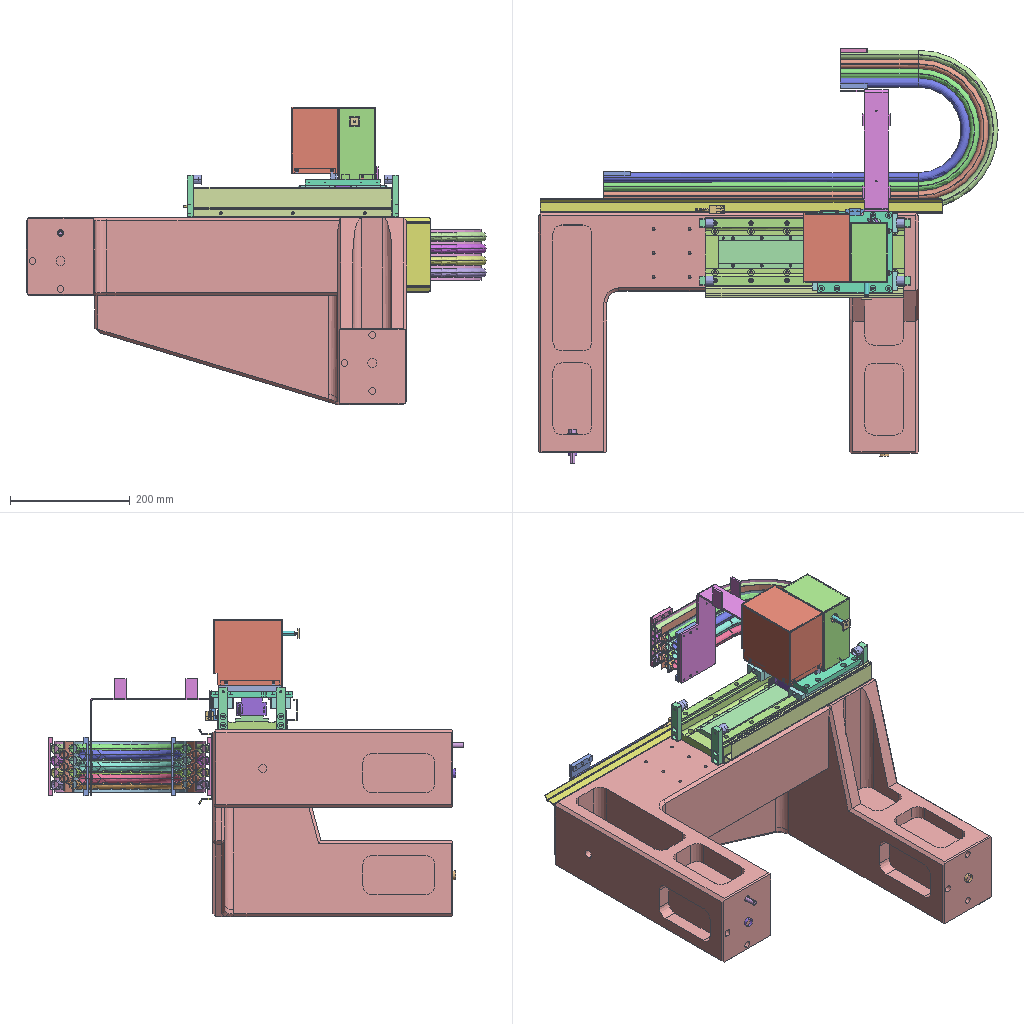Assembly | STEP file | 70 different items | 103 placed | box 767 x 693 x 496 mm
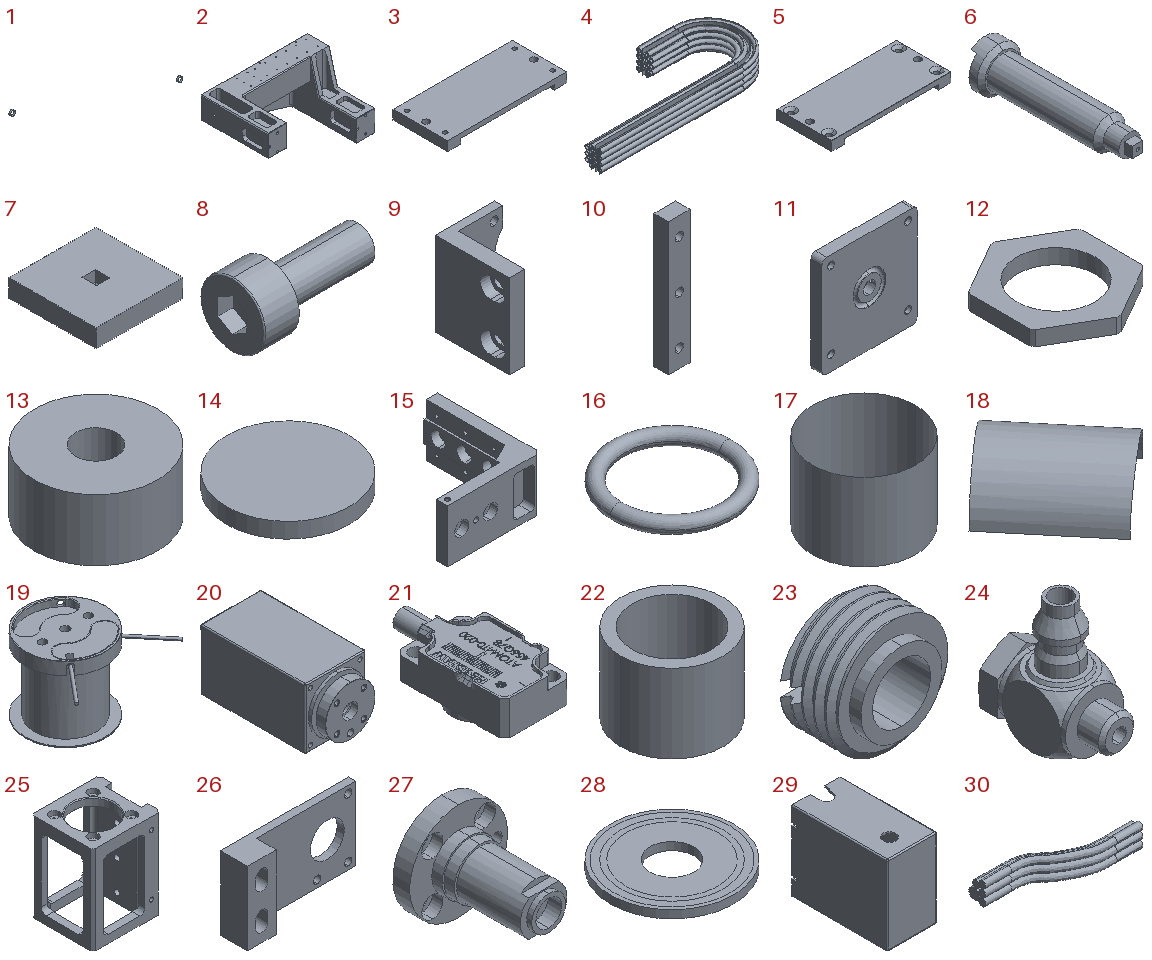Parts list (item | name | quantity | size | volume):
1 | COMPOUND | x1 | - | -
2 | SOLID | x1 | 635 x 400 x 312 mm | 15425228 mm3
3 | - | x2 | 97.7 x 44.7 x 7.7 mm | 19346 mm3
4 | - | x1 | 658 x 266 x 85.182 mm | 995637 mm3
5 | - | x2 | 97.7 x 44.7 x 7.7 mm | 18958 mm3
6 | - | x1 | 11 x 38.5 x 11 mm | 1504 mm3
7 | - | x1 | 16 x 16 x 3.3 mm | 788.101 mm3
8 | - | x1 | 11 x 5.5 x 5.5 mm | 120.454 mm3
9 | - | x1 | 14.8 x 18.5 x 21 mm | 1569 mm3
10 | - | x2 | 9 x 6 x 55 mm | 2652 mm3
11 | - | x1 | 39 x 10 x 41.5 mm | 7133 mm3
12 | - | x1 | 15 x 17 x 2 mm | 215.987 mm3
13 | - | x1 | 6 x 6 x 3 mm | 75.398 mm3
14 | - | x1 | 8 x 8 x 1 mm | 50.265 mm3
15 | - | x1 | 65 x 72 x 37 mm | 34772 mm3
16 | SOLID | x2 | 13 x 13 x 1.5 mm | 63.844 mm3
17 | SHELL | x2 | - | -
18 | SHELL | x1 | - | -
19 | COMPOUND | x1 | 48.485 x 46.549 x 32.7 mm | 5431 mm3
20 | - | x1 | 33.5 x 64.5 x 28 mm | 32538 mm3
21 | - | x2 | 12.7 x 25.5 x 7.883 mm | 1498 mm3
22 | - | x1 | 34.7 x 34.7 x 26.7 mm | 9963 mm3
23 | - | x1 | 10 x 5.5 x 10 mm | 234.976 mm3
24 | - | x1 | 5 x 9.5 x 10.687 mm | 200.166 mm3
25 | - | x1 | 40.5 x 37 x 53 mm | 18902 mm3
26 | - | x1 | 35.7 x 7.55 x 20.5 mm | 1672 mm3
27 | - | x1 | 23 x 27.7 x 23 mm | 2922 mm3
28 | - | x1 | 35.9 x 35.9 x 2.3 mm | 2028 mm3
29 | - | x1 | 62 x 120 x 99.5 mm | 84647 mm3
30 | - | x1 | 75 x 25.743 x 13 mm | 6214 mm3
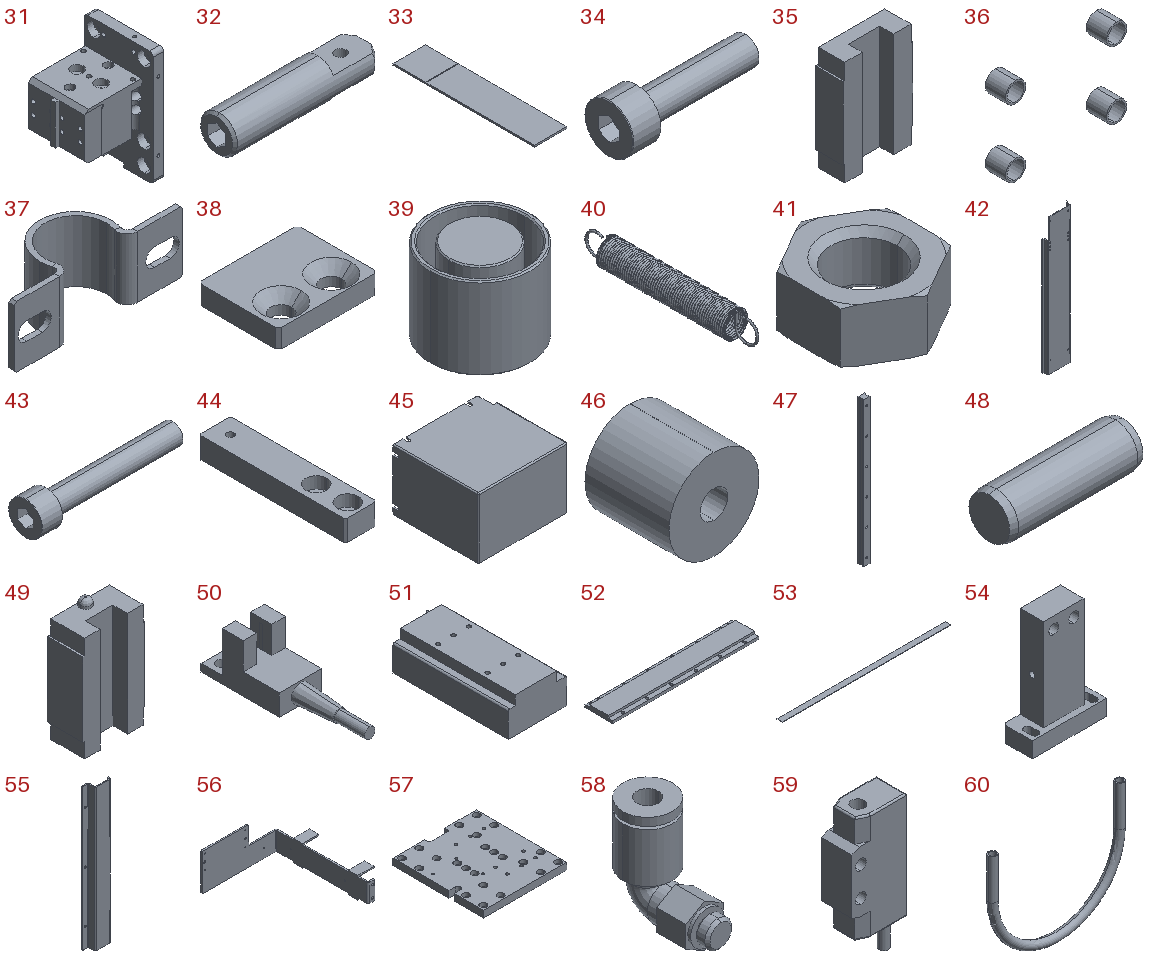31 | - | x1 | 59.1 x 57.6 x 95 mm | 75774 mm3
32 | - | x2 | 16 x 4 x 4 mm | 166.849 mm3
33 | - | x1 | 8 x 35 x 0.41 mm | 114.776 mm3
34 | - | x1 | 20 x 7 x 7 mm | 338.493 mm3
35 | SOLID | x2 | 20 x 8 x 30 mm | 3476 mm3
36 | COMPOUND | x2 | - | -
37 | - | x1 | 33 x 11.5 x 12 mm | 535.489 mm3
38 | - | x1 | 16 x 13 x 3 mm | 534.563 mm3
39 | - | x1 | 40 x 40 x 32.7 mm | 26304 mm3
40 | - | x2 | 6 x 40.5 x 6 mm | 206.632 mm3
41 | - | x2 | 6.649 x 7.66 x 3.2 mm | 79.578 mm3
42 | - | x1 | 125.321 x 23.845 x 670 mm | 206650 mm3
43 | - | x1 | 58 x 13 x 13 mm | 3445 mm3
44 | - | x4 | 15 x 70 x 10 mm | 9387 mm3
45 | - | x1 | 115 x 110 x 78 mm | 71850 mm3
46 | - | x4 | 15 x 14 x 15 mm | 1932 mm3
47 | - | x2 | 15 x 12.5 x 330 mm | 52950 mm3
48 | - | x6 | 12 x 4 x 4 mm | 149.498 mm3
49 | - | x4 | 34 x 19.5 x 65 mm | 29765 mm3
50 | - | x1 | 14 x 49 x 16 mm | 2990 mm3
51 | - | x1 | 50 x 113 x 30 mm | 135231 mm3
52 | - | x1 | 288 x 55 x 9.4 mm | 124869 mm3
53 | - | x1 | 235 x 8 x 0.5 mm | 940 mm3
54 | - | x1 | 33 x 13 x 48 mm | 9695 mm3
55 | - | x1 | 49.5 x 19 x 330 mm | 45387 mm3
56 | - | x1 | 195 x 202 x 83 mm | 64728 mm3
57 | - | x1 | 125 x 136 x 10 mm | 154591 mm3
58 | - | x8 | 9.3 x 18.35 x 19.641 mm | 1123 mm3
59 | - | x1 | 18 x 10 x 45 mm | 5334 mm3
60 | - | x1 | 67.5 x 4 x 53.75 mm | 768.291 mm3
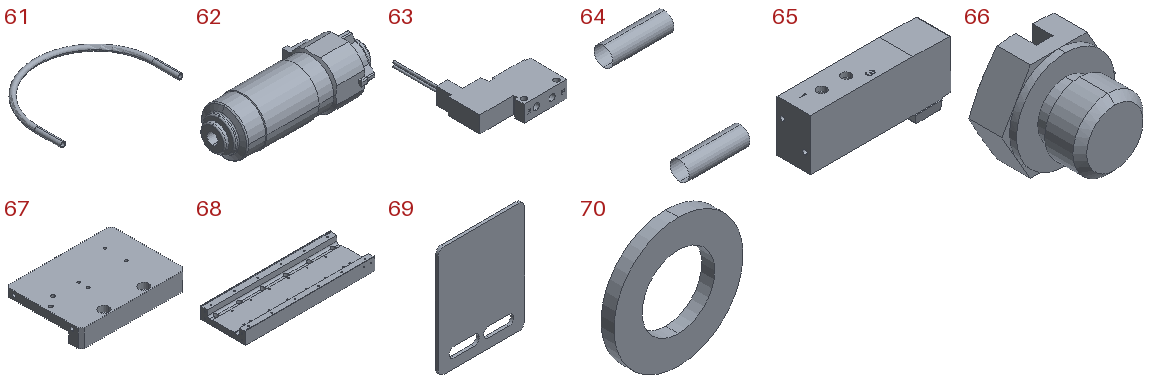61 | - | x1 | 94.3 x 67.15 x 4 mm | 999.734 mm3
62 | - | x1 | 53.9 x 23.5 x 18 mm | 11445 mm3
63 | - | x1 | 49.5 x 69.5 x 11 mm | 13145 mm3
64 | COMPOUND | x1 | - | -
65 | COMPOUND | x1 | 63 x 15 x 27.5 mm | 21811 mm3
66 | - | x1 | 8.083 x 6.5 x 7 mm | 172.44 mm3
67 | - | x1 | 105 x 75 x 18 mm | 73147 mm3
68 | - | x1 | 332 x 115 x 32 mm | 511026 mm3
69 | - | x1 | 30 x 1 x 38.5 mm | 1083 mm3
70 | - | x1 | 16 x 1.6 x 16 mm | 219.911 mm3
Placements (level | parent | child | x y z in mm | rotation matrix by rows):
1 | subassembly 2 | subassembly 3 | 0.0 -130.0 -72.5 | 1 0 0 0 1 0 0 0 1
2 | subassembly 3 | COMPOUND | 0.0 0.0 0.0 | 1 0 0 0 1 0 0 0 1
2 | subassembly 3 | SOLID | 0.0 0.0 0.0 | 1 0 0 0 1 0 0 0 1
1 | subassembly 2 | subassembly 4 | -526.0 28.45 -61.65 | -1 0 0 0 -1 0 0 0 1
2 | subassembly 4 | subassembly 5 | -417.35 -186.75 0.0 | 0 1 0 0 0 1 1 0 0
2 | subassembly 4 | subassembly 6 | 0.0 0.0 -0.0 | -1 0 0 0 -1 0 0 0 1
2 | subassembly 4 | subassembly 7 | -22.35 18.75 -0.0 | 0 -1 0 0 0 1 -1 0 0
2 | subassembly 4 | subassembly 7 | -417.35 -238.75 0.0 | 0 1 0 0 0 -1 -1 0 0
2 | subassembly 4 | subassembly 5 | -22.35 -33.25 -0.0 | 0 1 0 0 0 -1 -1 0 0
1 | subassembly 2 | subassembly 8 | -93.562 -1.69 180.388 | 1 0 0 0 -1 0 0 0 -1
2 | subassembly 8 | subassembly 9 | -22.044 8.453 6.73 | 0 1 0 0 0 1 1 0 0
3 | subassembly 9 | subassembly 10 | 13.608 28.356 133.257 | 1 0 0 0 0 1 0 -1 0
3 | subassembly 9 | subassembly 11 | 13.608 28.356 134.557 | 1 0 0 0 -1 0 0 0 -1
3 | subassembly 9 | subassembly 12 | 96.609 50.356 80.057 | 0 -0.6937 0.7203 -1 0 0 0 -0.7203 -0.6937
3 | subassembly 9 | subassembly 13 | 31.788 28.356 78.857 | -1 0 0 0 0 1 0 1 0
3 | subassembly 9 | subassembly 14 | 46.608 40.356 39.557 | 0 1 0 -1 0 0 0 0 1
3 | subassembly 9 | subassembly 15 | 13.608 28.356 16.557 | 0 0 -1 1 0 0 0 -1 0
3 | subassembly 9 | subassembly 16 | 13.608 28.356 78.357 | 0.8669 0.4986 0 -0.4986 0.8669 0 0 0 1
3 | subassembly 9 | subassembly 17 | 13.608 28.356 94.057 | 1 0 0 0 1 0 0 0 1
3 | subassembly 9 | subassembly 18 | 13.608 28.356 12.057 | 1 0 0 0 1 0 0 0 1
3 | subassembly 9 | subassembly 19 | 35.608 28.356 84.057 | -1 0 0 0 0 -1 0 -1 0
3 | subassembly 9 | subassembly 20 | 18.608 28.356 15.807 | 1 0 0 0 1 0 0 0 1
4 | subassembly 20 | SOLID | 0.0 0.0 0.0 | 1 0 0 0 1 0 0 0 1
4 | subassembly 20 | SHELL | 0.0 0.0 0.0 | 1 0 0 0 1 0 0 0 1
3 | subassembly 9 | subassembly 21 | 80.609 28.356 43.857 | -1 0 0 0 -1 0 0 0 1
4 | subassembly 21 | SHELL | 0.0 0.0 0.0 | 1 0 0 0 1 0 0 0 1
4 | subassembly 21 | COMPOUND | 0.0 0.0 0.0 | 1 0 0 0 1 0 0 0 1
3 | subassembly 9 | subassembly 22 | 13.608 28.356 65.057 | 0 0 -1 1 0 0 0 -1 0
3 | subassembly 9 | subassembly 23 | 58.608 54.406 51.807 | 1 0 0 0 0 1 0 -1 0
3 | subassembly 9 | subassembly 24 | 80.609 28.356 44.357 | 1 0 0 0 1 0 0 0 1
3 | subassembly 9 | subassembly 25 | 13.608 28.356 12.057 | 1 0 0 0 0 1 0 -1 0
3 | subassembly 9 | subassembly 26 | 13.608 47.856 14.307 | 0 0 1 0 1 0 -1 0 0
3 | subassembly 9 | subassembly 27 | 13.608 28.356 16.557 | 1 0 0 0 1 0 0 0 1
3 | subassembly 9 | subassembly 28 | 43.608 46.856 41.557 | 1 0 0 0 1 0 0 0 1
3 | subassembly 9 | subassembly 29 | 13.608 28.356 97.257 | -1 0 0 0 0 -1 0 -1 0
3 | subassembly 9 | subassembly 20 | 8.99 26.441 72.807 | -0.9237 -0.383 0 -0.383 0.9237 0 0 0 -1
4 | subassembly 20 | SOLID | 0.0 0.0 0.0 | 1 0 0 0 1 0 0 0 1
4 | subassembly 20 | SHELL | 0.0 0.0 0.0 | 1 0 0 0 1 0 0 0 1
3 | subassembly 9 | subassembly 23 | 33.639 38.606 80.857 | -1 0 0 0 -1 0 0 0 1
3 | subassembly 9 | subassembly 30 | 13.608 28.356 76.057 | 1 0 0 0 1 0 0 0 1
3 | subassembly 9 | subassembly 14 | 46.608 16.356 39.557 | 0 1 0 1 0 0 0 0 -1
2 | subassembly 8 | subassembly 31 | 10.762 114.309 56.388 | 1 0 0 0 0 -1 0 1 0
2 | subassembly 8 | subassembly 32 | 34.215 25.509 35.93 | -0.2588 0 -0.9659 0 1 0 0.9659 0 -0.2588
2 | subassembly 8 | subassembly 33 | -0.9952 36.963 55.888 | 1 0 0 0 1 0 0 0 1
3 | subassembly 33 | subassembly 34 | 7.307 41.846 31.45 | 0 -1 0 0 0 -1 1 0 0
3 | subassembly 33 | subassembly 35 | 27.857 -3.154 47.5 | 0 1 0 1 0 0 0 0 -1
3 | subassembly 33 | subassembly 36 | 30.457 22.346 14.4 | 0 0 1 0 -1 0 1 0 0
3 | subassembly 33 | subassembly 37 | -7.243 51.846 11.9 | 0 1 0 -1 0 0 0 0 1
3 | subassembly 33 | subassembly 38 | 19.307 22.346 -3.6 | 1 0 0 0 0 -1 0 1 0
4 | subassembly 38 | SOLID | 0.0 0.0 0.0 | 1 0 0 0 1 0 0 0 1
4 | subassembly 38 | COMPOUND | 0.0 0.0 0.0 | 1 0 0 0 1 0 0 0 1
3 | subassembly 33 | subassembly 39 | 11.557 -12.654 52 | 1 0 0 0 0 1 0 -1 0
3 | subassembly 33 | subassembly 40 | 7.307 71.346 53.291 | 0.9999 -0.0101 0 0 0 1 -0.0101 -0.9999 0
3 | subassembly 33 | subassembly 41 | 7.307 9.846 31.45 | 0 1 0 0 0 1 1 0 0
3 | subassembly 33 | subassembly 42 | 27.857 15.183 47.5 | 1 0 0 0 1 0 0 0 1
3 | subassembly 33 | subassembly 43 | 27.857 2.846 47.5 | 1 0 0 0 0 -1 0 1 0
3 | subassembly 33 | subassembly 35 | -13.143 -3.154 47.5 | 0 1 0 1 0 0 0 0 -1
3 | subassembly 33 | subassembly 42 | -13.143 15.183 47.5 | 1 0 0 0 1 0 0 0 1
3 | subassembly 33 | subassembly 38 | -4.693 22.346 -3.6 | 1 0 0 0 0 -1 0 1 0
4 | subassembly 38 | SOLID | 0.0 0.0 0.0 | 1 0 0 0 1 0 0 0 1
4 | subassembly 38 | COMPOUND | 0.0 0.0 0.0 | 1 0 0 0 1 0 0 0 1
3 | subassembly 33 | subassembly 43 | -13.143 2.846 47.5 | 1 0 0 0 0 -1 0 1 0
1 | subassembly 2 | subassembly 44 | -296.0 20.0 -6.65 | 0 0 -1 0 1 0 1 0 0
1 | subassembly 2 | subassembly 45 | -577.5 -360.4 -26.0 | 0 -0.9864 0.1642 -1 0 0 0 -0.1642 -0.9864
1 | subassembly 2 | subassembly 46 | 106.316 -53.777 125.223 | -1 0 0 0 0 1 0 1 0
2 | subassembly 46 | subassembly 47 | 462.316 -89.723 -59.223 | 0 0 1 0 1 0 -1 0 0
2 | subassembly 46 | subassembly 48 | 221.316 3.777 -4.723 | 0 0 1 0 -1 0 1 0 0
2 | subassembly 46 | subassembly 47 | 130.316 -89.723 36.777 | 0 0 -1 0 1 0 1 0 0
2 | subassembly 46 | subassembly 49 | 130.316 -62.223 36.777 | 0 1 0 -1 0 0 0 0 1
2 | subassembly 46 | subassembly 50 | 296.316 -97.223 -59.223 | 0 0 1 0 1 0 -1 0 0
2 | subassembly 46 | subassembly 49 | 130.316 -62.223 -59.223 | 0 1 0 -1 0 0 0 0 1
2 | subassembly 46 | subassembly 51 | 189.316 -67.593 -49.723 | 0 -1 0 1 0 0 0 0 1
2 | subassembly 46 | subassembly 52 | 255.816 -90.723 36.777 | 0 0 1 0 1 0 -1 0 0
2 | subassembly 46 | subassembly 49 | 462.316 -62.223 36.777 | 0 -1 0 1 0 0 0 0 1
2 | subassembly 46 | subassembly 53 | 440.316 -110.223 59.277 | 0 -1 0 0 0 1 -1 0 0
2 | subassembly 46 | subassembly 54 | 212.816 -86.223 -11.223 | 0 1 0 0 0 1 1 0 0
2 | subassembly 46 | subassembly 55 | 296.316 -108.723 -11.223 | -1 0 0 0 0 1 0 1 0
2 | subassembly 46 | subassembly 47 | 130.316 -89.723 -59.223 | 0 0 -1 0 1 0 1 0 0
2 | subassembly 46 | subassembly 56 | 297.316 -116.223 46.277 | 1 0 0 0 1 0 0 0 1
2 | subassembly 46 | subassembly 52 | 169.816 -90.723 36.777 | 0 0 1 0 1 0 -1 0 0
2 | subassembly 46 | subassembly 49 | 462.316 -62.223 -59.223 | 0 -1 0 1 0 0 0 0 1
2 | subassembly 46 | subassembly 57 | 210.016 -140.057 7.87 | 1 0 0 0 1 0 0 0 1
3 | subassembly 57 | subassembly 58 | 2.8 30.834 45.907 | -1 0 0 0 0 1 0 1 0
2 | subassembly 46 | subassembly 47 | 462.316 -89.723 36.777 | 0 0 1 0 1 0 -1 0 0
2 | subassembly 46 | subassembly 51 | 264.316 -64.752 -40.223 | 0 1 0 -1 0 0 0 0 1
2 | subassembly 46 | subassembly 59 | 296.316 -108.723 -68.723 | 0 0 1 1 0 0 0 1 0
2 | subassembly 46 | subassembly 60 | 197.316 -75.723 56.777 | 0 0 1 1 0 0 0 1 0
2 | subassembly 46 | subassembly 51 | 189.316 -67.593 27.277 | 0 -1 0 1 0 0 0 0 1
2 | subassembly 46 | subassembly 52 | 169.816 -90.723 -59.223 | 0 0 1 0 1 0 -1 0 0
2 | subassembly 46 | subassembly 61 | 212.816 -71.223 -11.223 | -1 0 0 0 0 1 0 1 0
2 | subassembly 46 | subassembly 51 | 178.316 -64.752 -40.223 | 0 1 0 -1 0 0 0 0 1
2 | subassembly 46 | subassembly 50 | 296.316 -97.223 36.777 | 0 0 1 0 1 0 -1 0 0
2 | subassembly 46 | subassembly 62 | 172.13 -58.938 5.965 | 0 1 0 0 0 1 1 0 0
3 | subassembly 62 | subassembly 63 | -56.188 90.187 28.215 | 0.6428 0 0.766 0 1 0 -0.766 0 0.6428
3 | subassembly 62 | subassembly 63 | 19.312 102.687 21.215 | 0 1 0 -1 0 0 0 0 1
3 | subassembly 62 | subassembly 64 | -33.438 87.687 20.715 | -1 0 0 0 0 1 0 1 0
3 | subassembly 62 | subassembly 63 | -54.188 67.187 31.715 | -1 0 0 0 -1 0 0 0 1
3 | subassembly 62 | subassembly 65 | 0.156 111.992 31.815 | -0.9561 0.2931 0 0.2931 0.9561 0 0 0 -1
3 | subassembly 62 | subassembly 66 | -11.834 71.627 34.615 | 0.9381 0 0.3464 0.3464 0 -0.9381 0 1 0
3 | subassembly 62 | subassembly 63 | -56.188 90.187 39.215 | 1 0 0 0 1 0 0 0 1
3 | subassembly 62 | subassembly 67 | -32.12 58.987 77.032 | -0.03428 0.9034 -0.4274 0 0.4277 0.9039 0.9994 0.03099 -0.01466
3 | subassembly 62 | subassembly 68 | 19.312 99.187 21.215 | 0 -1 0 1 0 0 0 0 1
3 | subassembly 62 | subassembly 69 | -56.188 78.687 47.215 | 0 1 0 0 0 1 1 0 0
4 | subassembly 69 | COMPOUND | 0.0 0.0 0.0 | 1 0 0 0 1 0 0 0 1
4 | subassembly 69 | COMPOUND | 0.0 0.0 0.0 | 1 0 0 0 1 0 0 0 1
3 | subassembly 62 | subassembly 63 | -30.188 70.187 20.715 | -0.9994 0 -0.03428 0 -1 0 -0.03428 0 0.9994
3 | subassembly 62 | subassembly 63 | -6.188 94.387 21.215 | 0 -1 0 0.9998 0 0.01843 -0.01843 0 0.9998
3 | subassembly 62 | subassembly 63 | 19.312 92.287 21.215 | 0 1 0 -1 0 0 0 0 1
3 | subassembly 62 | subassembly 63 | -30.188 105.187 20.715 | 1 0 0 0 1 0 0 0 1
3 | subassembly 62 | subassembly 70 | -2.688 104.987 21.215 | 0 -1 0 0.8372 0 0.5469 -0.5469 0 0.8372
3 | subassembly 62 | subassembly 71 | -13.688 87.687 7.715 | 1 0 0 0 1 0 0 0 1
2 | subassembly 46 | subassembly 51 | 161.316 -64.752 -40.223 | 0 1 0 -1 0 0 0 0 1
2 | subassembly 46 | subassembly 72 | 296.316 -125.223 -11.223 | 1 0 0 0 0 1 0 -1 0
2 | subassembly 46 | subassembly 73 | 255.816 -61.223 56.777 | -1 0 0 0 0 -1 0 -1 0
2 | subassembly 46 | subassembly 51 | 247.316 -64.752 -40.223 | 0 1 0 -1 0 0 0 0 1
2 | subassembly 46 | subassembly 52 | 255.816 -90.723 -59.223 | 0 0 1 0 1 0 -1 0 0
1 | subassembly 2 | subassembly 74 | -577.5 -378.644 -26.0 | 0.9156 0 0.4021 0 1 0 -0.4021 0 0.9156